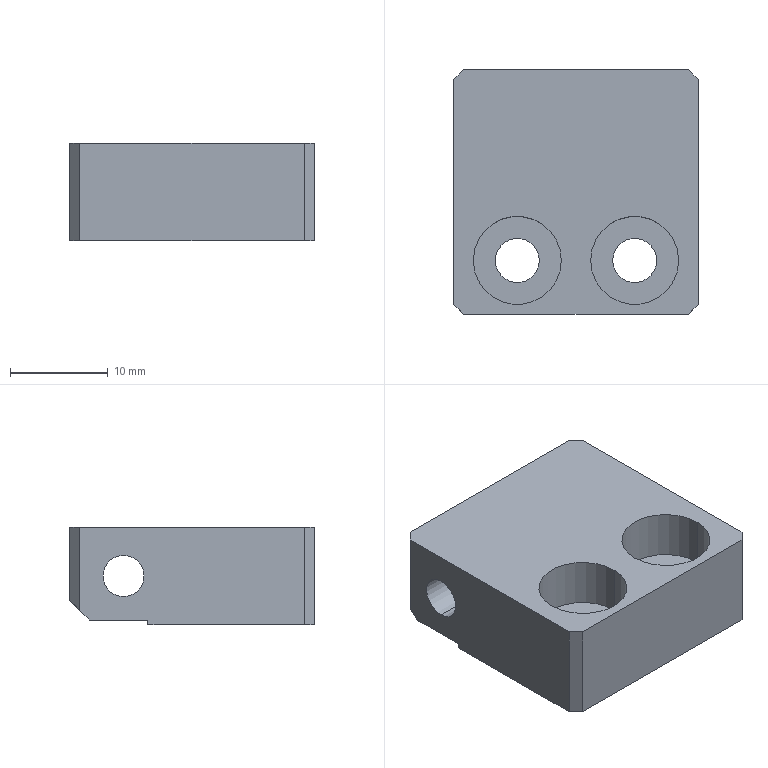Part | SolidWorks | features ICE 4, Chamfer 2, 3DProfileFeature 1, Extrusion 1, HoleWzd 1 | 1 solid | 25 faces | box 25 x 25 x 10 mm | volume 4941 mm3 | plane 15 | cylinder 10 | commonest cylinder face diameters 4.5 x4 9 x4 4.2 x2
STEP:
#1=CARTESIAN_POINT('',(12.5,7.,2.9));
#2=VERTEX_POINT('',#1);
#3=CARTESIAN_POINT('',(12.5,7.,7.1));
#4=VERTEX_POINT('',#3);
#5=CARTESIAN_POINT('',(12.5,7.,5.));
#6=DIRECTION('',(-1.,0.,0.));
#7=DIRECTION('',(0.,0.,1.));
#8=AXIS2_PLACEMENT_3D('',#5,#6,#7);
#9=CIRCLE('',#8,2.1);
#10=EDGE_CURVE('',#2,#4,#9,.T.);
#11=ORIENTED_EDGE('',*,*,#10,.F.);
#12=CARTESIAN_POINT('',(-12.5,7.,2.9));
#13=VERTEX_POINT('',#12);
#14=CARTESIAN_POINT('',(-12.5,7.,2.9));
#15=DIRECTION('',(-1.,0.,0.));
#16=VECTOR('',#15,1000.);
#17=LINE('',#14,#16);
#18=EDGE_CURVE('',#2,#13,#17,.T.);
#19=ORIENTED_EDGE('',*,*,#18,.T.);
#20=CARTESIAN_POINT('',(-12.5,7.,7.1));
#21=VERTEX_POINT('',#20);
#22=CARTESIAN_POINT('',(-12.5,7.,5.));
#23=DIRECTION('',(-1.,0.,0.));
#24=DIRECTION('',(0.,0.,1.));
#25=AXIS2_PLACEMENT_3D('',#22,#23,#24);
#26=CIRCLE('',#25,2.1);
#27=EDGE_CURVE('',#13,#21,#26,.T.);
#28=ORIENTED_EDGE('',*,*,#27,.T.);
#29=CARTESIAN_POINT('',(-12.5,7.,7.1));
#30=DIRECTION('',(-1.,0.,0.));
#31=VECTOR('',#30,1000.);
#32=LINE('',#29,#31);
#33=EDGE_CURVE('',#4,#21,#32,.T.);
#34=ORIENTED_EDGE('',*,*,#33,.F.);
#35=EDGE_LOOP('',(#11,#19,#28,#34));
#36=FACE_OUTER_BOUND('',#35,.T.);
#37=CARTESIAN_POINT('',(-12.5,7.,5.));
#38=DIRECTION('',(-1.,0.,0.));
#39=DIRECTION('',(0.,0.,1.));
#40=AXIS2_PLACEMENT_3D('',#37,#38,#39);
#41=CYLINDRICAL_SURFACE('',#40,2.1);
#42=ADVANCED_FACE('',(#36),#41,.F.);
#43=CARTESIAN_POINT('',(3.75,-7.,0.));
#44=VERTEX_POINT('',#43);
#45=CARTESIAN_POINT('',(8.25,-7.,0.));
#46=VERTEX_POINT('',#45);
#47=CARTESIAN_POINT('',(6.,-7.,0.));
#48=DIRECTION('',(0.,0.,1.));
#49=DIRECTION('',(1.,0.,0.));
#50=AXIS2_PLACEMENT_3D('',#47,#48,#49);
#51=CIRCLE('',#50,2.25);
#52=EDGE_CURVE('',#44,#46,#51,.T.);
#53=ORIENTED_EDGE('',*,*,#52,.F.);
#54=CARTESIAN_POINT('',(3.75,-7.,5.));
#55=VERTEX_POINT('',#54);
#56=CARTESIAN_POINT('',(3.75,-7.,-4.));
#57=DIRECTION('',(0.,0.,1.));
#58=VECTOR('',#57,1000.);
#59=LINE('',#56,#58);
#60=EDGE_CURVE('',#44,#55,#59,.T.);
#61=ORIENTED_EDGE('',*,*,#60,.T.);
#62=CARTESIAN_POINT('',(8.25,-7.,5.));
#63=VERTEX_POINT('',#62);
#64=CARTESIAN_POINT('',(6.,-7.,5.));
#65=DIRECTION('',(0.,0.,-1.));
#66=DIRECTION('',(-1.,0.,0.));
#67=AXIS2_PLACEMENT_3D('',#64,#65,#66);
#68=CIRCLE('',#67,2.25);
#69=EDGE_CURVE('',#63,#55,#68,.T.);
#70=ORIENTED_EDGE('',*,*,#69,.F.);
#71=CARTESIAN_POINT('',(8.25,-7.,-4.));
#72=DIRECTION('',(0.,0.,1.));
#73=VECTOR('',#72,1000.);
#74=LINE('',#71,#73);
#75=EDGE_CURVE('',#46,#63,#74,.T.);
#76=ORIENTED_EDGE('',*,*,#75,.F.);
#77=EDGE_LOOP('',(#53,#61,#70,#76));
#78=FACE_OUTER_BOUND('',#77,.T.);
#79=CARTESIAN_POINT('',(6.,-7.,-4.));
#80=DIRECTION('',(0.,0.,1.));
#81=DIRECTION('',(1.,0.,0.));
#82=AXIS2_PLACEMENT_3D('',#79,#80,#81);
#83=CYLINDRICAL_SURFACE('',#82,2.25);
#84=ADVANCED_FACE('',(#78),#83,.F.);
#85=CARTESIAN_POINT('',(-8.25,-7.,0.));
#86=VERTEX_POINT('',#85);
#87=CARTESIAN_POINT('',(-3.75,-7.,0.));
#88=VERTEX_POINT('',#87);
#89=CARTESIAN_POINT('',(-6.,-7.,0.));
#90=DIRECTION('',(0.,0.,1.));
#91=DIRECTION('',(1.,0.,0.));
#92=AXIS2_PLACEMENT_3D('',#89,#90,#91);
#93=CIRCLE('',#92,2.25);
#94=EDGE_CURVE('',#86,#88,#93,.T.);
#95=ORIENTED_EDGE('',*,*,#94,.F.);
#96=CARTESIAN_POINT('',(-8.25,-7.,5.));
#97=VERTEX_POINT('',#96);
#98=CARTESIAN_POINT('',(-8.25,-7.,-4.));
#99=DIRECTION('',(0.,0.,1.));
#100=VECTOR('',#99,1000.);
#101=LINE('',#98,#100);
#102=EDGE_CURVE('',#86,#97,#101,.T.);
#103=ORIENTED_EDGE('',*,*,#102,.T.);
#104=CARTESIAN_POINT('',(-3.75,-7.,5.));
#105=VERTEX_POINT('',#104);
#106=CARTESIAN_POINT('',(-6.,-7.,5.));
#107=DIRECTION('',(0.,0.,1.));
#108=DIRECTION('',(1.,0.,0.));
#109=AXIS2_PLACEMENT_3D('',#106,#107,#108);
#110=CIRCLE('',#109,2.25);
#111=EDGE_CURVE('',#97,#105,#110,.T.);
#112=ORIENTED_EDGE('',*,*,#111,.T.);
#113=CARTESIAN_POINT('',(-3.75,-7.,-4.));
#114=DIRECTION('',(0.,0.,1.));
#115=VECTOR('',#114,1000.);
#116=LINE('',#113,#115);
#117=EDGE_CURVE('',#88,#105,#116,.T.);
#118=ORIENTED_EDGE('',*,*,#117,.F.);
#119=EDGE_LOOP('',(#95,#103,#112,#118));
#120=FACE_OUTER_BOUND('',#119,.T.);
#121=CARTESIAN_POINT('',(-6.,-7.,-4.));
#122=DIRECTION('',(0.,0.,1.));
#123=DIRECTION('',(1.,0.,0.));
#124=AXIS2_PLACEMENT_3D('',#121,#122,#123);
#125=CYLINDRICAL_SURFACE('',#124,2.25);
#126=ADVANCED_FACE('',(#120),#125,.F.);
#127=CARTESIAN_POINT('',(1.5,-7.,5.));
#128=VERTEX_POINT('',#127);
#129=CARTESIAN_POINT('',(10.5,-7.,5.));
#130=VERTEX_POINT('',#129);
#131=CARTESIAN_POINT('',(6.,-7.,5.));
#132=DIRECTION('',(0.,0.,1.));
#133=DIRECTION('',(-1.,0.,0.));
#134=AXIS2_PLACEMENT_3D('',#131,#132,#133);
#135=CIRCLE('',#134,4.5);
#136=EDGE_CURVE('',#128,#130,#135,.T.);
#137=ORIENTED_EDGE('',*,*,#136,.F.);
#138=CARTESIAN_POINT('',(1.5,-7.,10.));
#139=VERTEX_POINT('',#138);
#140=CARTESIAN_POINT('',(1.5,-7.,5.));
#141=DIRECTION('',(0.,0.,1.));
#142=VECTOR('',#141,1000.);
#143=LINE('',#140,#142);
#144=EDGE_CURVE('',#128,#139,#143,.T.);
#145=ORIENTED_EDGE('',*,*,#144,.T.);
#146=CARTESIAN_POINT('',(10.5,-7.,10.));
#147=VERTEX_POINT('',#146);
#148=CARTESIAN_POINT('',(6.,-7.,10.));
#149=DIRECTION('',(0.,0.,1.));
#150=DIRECTION('',(-1.,0.,0.));
#151=AXIS2_PLACEMENT_3D('',#148,#149,#150);
#152=CIRCLE('',#151,4.5);
#153=EDGE_CURVE('',#139,#147,#152,.T.);
#154=ORIENTED_EDGE('',*,*,#153,.T.);
#155=CARTESIAN_POINT('',(10.5,-7.,5.));
#156=DIRECTION('',(0.,0.,1.));
#157=VECTOR('',#156,1000.);
#158=LINE('',#155,#157);
#159=EDGE_CURVE('',#130,#147,#158,.T.);
#160=ORIENTED_EDGE('',*,*,#159,.F.);
#161=EDGE_LOOP('',(#137,#145,#154,#160));
#162=FACE_OUTER_BOUND('',#161,.T.);
#163=CARTESIAN_POINT('',(6.,-7.,5.));
#164=DIRECTION('',(0.,0.,1.));
#165=DIRECTION('',(1.,0.,0.));
#166=AXIS2_PLACEMENT_3D('',#163,#164,#165);
#167=CYLINDRICAL_SURFACE('',#166,4.5);
#168=ADVANCED_FACE('',(#162),#167,.F.);
#169=CARTESIAN_POINT('',(-10.5,-7.,5.));
#170=VERTEX_POINT('',#169);
#171=CARTESIAN_POINT('',(-1.5,-7.,5.));
#172=VERTEX_POINT('',#171);
#173=CARTESIAN_POINT('',(-6.,-7.,5.));
#174=DIRECTION('',(0.,0.,1.));
#175=DIRECTION('',(1.,0.,0.));
#176=AXIS2_PLACEMENT_3D('',#173,#174,#175);
#177=CIRCLE('',#176,4.5);
#178=EDGE_CURVE('',#170,#172,#177,.T.);
#179=ORIENTED_EDGE('',*,*,#178,.F.);
#180=CARTESIAN_POINT('',(-10.5,-7.,10.));
#181=VERTEX_POINT('',#180);
#182=CARTESIAN_POINT('',(-10.5,-7.,5.));
#183=DIRECTION('',(0.,0.,1.));
#184=VECTOR('',#183,1000.);
#185=LINE('',#182,#184);
#186=EDGE_CURVE('',#170,#181,#185,.T.);
#187=ORIENTED_EDGE('',*,*,#186,.T.);
#188=CARTESIAN_POINT('',(-1.5,-7.,10.));
#189=VERTEX_POINT('',#188);
#190=CARTESIAN_POINT('',(-6.,-7.,10.));
#191=DIRECTION('',(0.,0.,1.));
#192=DIRECTION('',(1.,0.,0.));
#193=AXIS2_PLACEMENT_3D('',#190,#191,#192);
#194=CIRCLE('',#193,4.5);
#195=EDGE_CURVE('',#181,#189,#194,.T.);
#196=ORIENTED_EDGE('',*,*,#195,.T.);
#197=CARTESIAN_POINT('',(-1.5,-7.,5.));
#198=DIRECTION('',(0.,0.,1.));
#199=VECTOR('',#198,1000.);
#200=LINE('',#197,#199);
#201=EDGE_CURVE('',#172,#189,#200,.T.);
#202=ORIENTED_EDGE('',*,*,#201,.F.);
#203=EDGE_LOOP('',(#179,#187,#196,#202));
#204=FACE_OUTER_BOUND('',#203,.T.);
#205=CARTESIAN_POINT('',(-6.,-7.,5.));
#206=DIRECTION('',(0.,0.,1.));
#207=DIRECTION('',(1.,0.,0.));
#208=AXIS2_PLACEMENT_3D('',#205,#206,#207);
#209=CYLINDRICAL_SURFACE('',#208,4.5);
#210=ADVANCED_FACE('',(#204),#209,.F.);
#211=CARTESIAN_POINT('',(12.5,7.,5.));
#212=DIRECTION('',(-1.,0.,0.));
#213=DIRECTION('',(0.,0.,1.));
#214=AXIS2_PLACEMENT_3D('',#211,#212,#213);
#215=CIRCLE('',#214,2.1);
#216=EDGE_CURVE('',#4,#2,#215,.T.);
#217=ORIENTED_EDGE('',*,*,#216,.T.);
#218=ORIENTED_EDGE('',*,*,#10,.T.);
#219=EDGE_LOOP('',(#217,#218));
#220=FACE_BOUND('',#219,.T.);
#221=CARTESIAN_POINT('',(12.5,4.5,0.5));
#222=VERTEX_POINT('',#221);
#223=CARTESIAN_POINT('',(12.5,10.5,0.5));
#224=VERTEX_POINT('',#223);
#225=CARTESIAN_POINT('',(12.5,12.5,0.5));
#226=DIRECTION('',(0.,1.,0.));
#227=VECTOR('',#226,1000.);
#228=LINE('',#225,#227);
#229=EDGE_CURVE('',#222,#224,#228,.T.);
#230=ORIENTED_EDGE('',*,*,#229,.T.);
#231=CARTESIAN_POINT('',(12.5,11.5,1.5));
#232=VERTEX_POINT('',#231);
#233=CARTESIAN_POINT('',(12.5,12.5,2.5));
#234=DIRECTION('',(0.,0.7071,0.7071));
#235=VECTOR('',#234,1000.);
#236=LINE('',#233,#235);
#237=EDGE_CURVE('',#224,#232,#236,.T.);
#238=ORIENTED_EDGE('',*,*,#237,.T.);
#239=CARTESIAN_POINT('',(12.5,11.5,10.));
#240=VERTEX_POINT('',#239);
#241=CARTESIAN_POINT('',(12.5,11.5,10.));
#242=DIRECTION('',(0.,0.,1.));
#243=VECTOR('',#242,1000.);
#244=LINE('',#241,#243);
#245=EDGE_CURVE('',#232,#240,#244,.T.);
#246=ORIENTED_EDGE('',*,*,#245,.T.);
#247=CARTESIAN_POINT('',(12.5,-11.5,10.));
#248=VERTEX_POINT('',#247);
#249=CARTESIAN_POINT('',(12.5,12.5,10.));
#250=DIRECTION('',(0.,1.,0.));
#251=VECTOR('',#250,1000.);
#252=LINE('',#249,#251);
#253=EDGE_CURVE('',#248,#240,#252,.T.);
#254=ORIENTED_EDGE('',*,*,#253,.F.);
#255=CARTESIAN_POINT('',(12.5,-11.5,0.));
#256=VERTEX_POINT('',#255);
#257=CARTESIAN_POINT('',(12.5,-11.5,10.));
#258=DIRECTION('',(0.,0.,-1.));
#259=VECTOR('',#258,1000.);
#260=LINE('',#257,#259);
#261=EDGE_CURVE('',#248,#256,#260,.T.);
#262=ORIENTED_EDGE('',*,*,#261,.T.);
#263=CARTESIAN_POINT('',(12.5,4.5,0.));
#264=VERTEX_POINT('',#263);
#265=CARTESIAN_POINT('',(12.5,12.5,0.));
#266=DIRECTION('',(0.,1.,0.));
#267=VECTOR('',#266,1000.);
#268=LINE('',#265,#267);
#269=EDGE_CURVE('',#256,#264,#268,.T.);
#270=ORIENTED_EDGE('',*,*,#269,.T.);
#271=CARTESIAN_POINT('',(12.5,4.5,10.));
#272=DIRECTION('',(0.,0.,1.));
#273=VECTOR('',#272,1000.);
#274=LINE('',#271,#273);
#275=EDGE_CURVE('',#264,#222,#274,.T.);
#276=ORIENTED_EDGE('',*,*,#275,.T.);
#277=EDGE_LOOP('',(#230,#238,#246,#254,#262,#270,#276));
#278=FACE_OUTER_BOUND('',#277,.T.);
#279=CARTESIAN_POINT('',(12.5,12.5,10.));
#280=DIRECTION('',(-1.,0.,0.));
#281=DIRECTION('',(0.,-1.,0.));
#282=AXIS2_PLACEMENT_3D('',#279,#280,#281);
#283=PLANE('',#282);
#284=ADVANCED_FACE('',(#220,#278),#283,.F.);
#285=CARTESIAN_POINT('',(11.5,12.5,10.));
#286=VERTEX_POINT('',#285);
#287=CARTESIAN_POINT('',(11.5,12.5,2.5));
#288=VERTEX_POINT('',#287);
#289=CARTESIAN_POINT('',(11.5,12.5,10.));
#290=DIRECTION('',(0.,0.,-1.));
#291=VECTOR('',#290,1000.);
#292=LINE('',#289,#291);
#293=EDGE_CURVE('',#286,#288,#292,.T.);
#294=ORIENTED_EDGE('',*,*,#293,.T.);
#295=CARTESIAN_POINT('',(-11.5,12.5,2.5));
#296=VERTEX_POINT('',#295);
#297=CARTESIAN_POINT('',(-12.5,12.5,2.5));
#298=DIRECTION('',(-1.,0.,0.));
#299=VECTOR('',#298,1000.);
#300=LINE('',#297,#299);
#301=EDGE_CURVE('',#288,#296,#300,.T.);
#302=ORIENTED_EDGE('',*,*,#301,.T.);
#303=CARTESIAN_POINT('',(-11.5,12.5,10.));
#304=VERTEX_POINT('',#303);
#305=CARTESIAN_POINT('',(-11.5,12.5,10.));
#306=DIRECTION('',(0.,0.,1.));
#307=VECTOR('',#306,1000.);
#308=LINE('',#305,#307);
#309=EDGE_CURVE('',#296,#304,#308,.T.);
#310=ORIENTED_EDGE('',*,*,#309,.T.);
#311=CARTESIAN_POINT('',(-12.5,12.5,10.));
#312=DIRECTION('',(-1.,0.,0.));
#313=VECTOR('',#312,1000.);
#314=LINE('',#311,#313);
#315=EDGE_CURVE('',#286,#304,#314,.T.);
#316=ORIENTED_EDGE('',*,*,#315,.F.);
#317=EDGE_LOOP('',(#294,#302,#310,#316));
#318=FACE_OUTER_BOUND('',#317,.T.);
#319=CARTESIAN_POINT('',(-12.5,12.5,10.));
#320=DIRECTION('',(0.,-1.,0.));
#321=DIRECTION('',(0.,0.,-1.));
#322=AXIS2_PLACEMENT_3D('',#319,#320,#321);
#323=PLANE('',#322);
#324=ADVANCED_FACE('',(#318),#323,.F.);
#325=CARTESIAN_POINT('',(-12.5,7.,5.));
#326=DIRECTION('',(-1.,0.,0.));
#327=DIRECTION('',(0.,0.,1.));
#328=AXIS2_PLACEMENT_3D('',#325,#326,#327);
#329=CIRCLE('',#328,2.1);
#330=EDGE_CURVE('',#21,#13,#329,.T.);
#331=ORIENTED_EDGE('',*,*,#330,.F.);
#332=ORIENTED_EDGE('',*,*,#27,.F.);
#333=EDGE_LOOP('',(#331,#332));
#334=FACE_BOUND('',#333,.T.);
#335=CARTESIAN_POINT('',(-12.5,11.5,10.));
#336=VERTEX_POINT('',#335);
#337=CARTESIAN_POINT('',(-12.5,11.5,1.5));
#338=VERTEX_POINT('',#337);
#339=CARTESIAN_POINT('',(-12.5,11.5,10.));
#340=DIRECTION('',(0.,0.,-1.));
#341=VECTOR('',#340,1000.);
#342=LINE('',#339,#341);
#343=EDGE_CURVE('',#336,#338,#342,.T.);
#344=ORIENTED_EDGE('',*,*,#343,.T.);
#345=CARTESIAN_POINT('',(-12.5,10.5,0.5));
#346=VERTEX_POINT('',#345);
#347=CARTESIAN_POINT('',(-12.5,12.5,2.5));
#348=DIRECTION('',(0.,-0.7071,-0.7071));
#349=VECTOR('',#348,1000.);
#350=LINE('',#347,#349);
#351=EDGE_CURVE('',#338,#346,#350,.T.);
#352=ORIENTED_EDGE('',*,*,#351,.T.);
#353=CARTESIAN_POINT('',(-12.5,4.5,0.5));
#354=VERTEX_POINT('',#353);
#355=CARTESIAN_POINT('',(-12.5,12.5,0.5));
#356=DIRECTION('',(0.,1.,0.));
#357=VECTOR('',#356,1000.);
#358=LINE('',#355,#357);
#359=EDGE_CURVE('',#354,#346,#358,.T.);
#360=ORIENTED_EDGE('',*,*,#359,.F.);
#361=CARTESIAN_POINT('',(-12.5,4.5,0.));
#362=VERTEX_POINT('',#361);
#363=CARTESIAN_POINT('',(-12.5,4.5,0.));
#364=DIRECTION('',(0.,0.,1.));
#365=VECTOR('',#364,1000.);
#366=LINE('',#363,#365);
#367=EDGE_CURVE('',#362,#354,#366,.T.);
#368=ORIENTED_EDGE('',*,*,#367,.F.);
#369=CARTESIAN_POINT('',(-12.5,-11.5,0.));
#370=VERTEX_POINT('',#369);
#371=CARTESIAN_POINT('',(-12.5,12.5,0.));
#372=DIRECTION('',(0.,-1.,0.));
#373=VECTOR('',#372,1000.);
#374=LINE('',#371,#373);
#375=EDGE_CURVE('',#362,#370,#374,.T.);
#376=ORIENTED_EDGE('',*,*,#375,.T.);
#377=CARTESIAN_POINT('',(-12.5,-11.5,10.));
#378=VERTEX_POINT('',#377);
#379=CARTESIAN_POINT('',(-12.5,-11.5,10.));
#380=DIRECTION('',(0.,0.,1.));
#381=VECTOR('',#380,1000.);
#382=LINE('',#379,#381);
#383=EDGE_CURVE('',#370,#378,#382,.T.);
#384=ORIENTED_EDGE('',*,*,#383,.T.);
#385=CARTESIAN_POINT('',(-12.5,12.5,10.));
#386=DIRECTION('',(0.,-1.,0.));
#387=VECTOR('',#386,1000.);
#388=LINE('',#385,#387);
#389=EDGE_CURVE('',#336,#378,#388,.T.);
#390=ORIENTED_EDGE('',*,*,#389,.F.);
#391=EDGE_LOOP('',(#344,#352,#360,#368,#376,#384,#390));
#392=FACE_OUTER_BOUND('',#391,.T.);
#393=CARTESIAN_POINT('',(-12.5,12.5,10.));
#394=DIRECTION('',(1.,0.,0.));
#395=DIRECTION('',(0.,1.,0.));
#396=AXIS2_PLACEMENT_3D('',#393,#394,#395);
#397=PLANE('',#396);
#398=ADVANCED_FACE('',(#334,#392),#397,.F.);
#399=CARTESIAN_POINT('',(-11.5,-12.5,0.));
#400=VERTEX_POINT('',#399);
#401=CARTESIAN_POINT('',(11.5,-12.5,0.));
#402=VERTEX_POINT('',#401);
#403=CARTESIAN_POINT('',(-12.5,-12.5,0.));
#404=DIRECTION('',(1.,0.,0.));
#405=VECTOR('',#404,1000.);
#406=LINE('',#403,#405);
#407=EDGE_CURVE('',#400,#402,#406,.T.);
#408=ORIENTED_EDGE('',*,*,#407,.T.);
#409=CARTESIAN_POINT('',(11.5,-12.5,10.));
#410=VERTEX_POINT('',#409);
#411=CARTESIAN_POINT('',(11.5,-12.5,10.));
#412=DIRECTION('',(0.,0.,1.));
#413=VECTOR('',#412,1000.);
#414=LINE('',#411,#413);
#415=EDGE_CURVE('',#402,#410,#414,.T.);
#416=ORIENTED_EDGE('',*,*,#415,.T.);
#417=CARTESIAN_POINT('',(-11.5,-12.5,10.));
#418=VERTEX_POINT('',#417);
#419=CARTESIAN_POINT('',(-12.5,-12.5,10.));
#420=DIRECTION('',(1.,0.,0.));
#421=VECTOR('',#420,1000.);
#422=LINE('',#419,#421);
#423=EDGE_CURVE('',#418,#410,#422,.T.);
#424=ORIENTED_EDGE('',*,*,#423,.F.);
#425=CARTESIAN_POINT('',(-11.5,-12.5,10.));
#426=DIRECTION('',(0.,0.,-1.));
#427=VECTOR('',#426,1000.);
#428=LINE('',#425,#427);
#429=EDGE_CURVE('',#418,#400,#428,.T.);
#430=ORIENTED_EDGE('',*,*,#429,.T.);
#431=EDGE_LOOP('',(#408,#416,#424,#430));
#432=FACE_OUTER_BOUND('',#431,.T.);
#433=CARTESIAN_POINT('',(-12.5,-12.5,10.));
#434=DIRECTION('',(0.,1.,0.));
#435=DIRECTION('',(0.,0.,1.));
#436=AXIS2_PLACEMENT_3D('',#433,#434,#435);
#437=PLANE('',#436);
#438=ADVANCED_FACE('',(#432),#437,.F.);
#439=CARTESIAN_POINT('',(6.,-7.,10.));
#440=DIRECTION('',(0.,0.,1.));
#441=DIRECTION('',(-1.,0.,0.));
#442=AXIS2_PLACEMENT_3D('',#439,#440,#441);
#443=CIRCLE('',#442,4.5);
#444=EDGE_CURVE('',#147,#139,#443,.T.);
#445=ORIENTED_EDGE('',*,*,#444,.F.);
#446=ORIENTED_EDGE('',*,*,#153,.F.);
#447=EDGE_LOOP('',(#445,#446));
#448=FACE_BOUND('',#447,.T.);
#449=CARTESIAN_POINT('',(-6.,-7.,10.));
#450=DIRECTION('',(0.,0.,1.));
#451=DIRECTION('',(1.,0.,0.));
#452=AXIS2_PLACEMENT_3D('',#449,#450,#451);
#453=CIRCLE('',#452,4.5);
#454=EDGE_CURVE('',#189,#181,#453,.T.);
#455=ORIENTED_EDGE('',*,*,#454,.F.);
#456=ORIENTED_EDGE('',*,*,#195,.F.);
#457=EDGE_LOOP('',(#455,#456));
#458=FACE_BOUND('',#457,.T.);
#459=ORIENTED_EDGE('',*,*,#423,.T.);
#460=CARTESIAN_POINT('',(12.,-12.,10.));
#461=DIRECTION('',(0.7071,0.7071,0.));
#462=VECTOR('',#461,1000.);
#463=LINE('',#460,#462);
#464=EDGE_CURVE('',#410,#248,#463,.T.);
#465=ORIENTED_EDGE('',*,*,#464,.T.);
#466=ORIENTED_EDGE('',*,*,#253,.T.);
#467=CARTESIAN_POINT('',(12.,12.,10.));
#468=DIRECTION('',(-0.7071,0.7071,0.));
#469=VECTOR('',#468,1000.);
#470=LINE('',#467,#469);
#471=EDGE_CURVE('',#240,#286,#470,.T.);
#472=ORIENTED_EDGE('',*,*,#471,.T.);
#473=ORIENTED_EDGE('',*,*,#315,.T.);
#474=CARTESIAN_POINT('',(-12.,12.,10.));
#475=DIRECTION('',(-0.7071,-0.7071,0.));
#476=VECTOR('',#475,1000.);
#477=LINE('',#474,#476);
#478=EDGE_CURVE('',#304,#336,#477,.T.);
#479=ORIENTED_EDGE('',*,*,#478,.T.);
#480=ORIENTED_EDGE('',*,*,#389,.T.);
#481=CARTESIAN_POINT('',(-12.,-12.,10.));
#482=DIRECTION('',(0.7071,-0.7071,0.));
#483=VECTOR('',#482,1000.);
#484=LINE('',#481,#483);
#485=EDGE_CURVE('',#378,#418,#484,.T.);
#486=ORIENTED_EDGE('',*,*,#485,.T.);
#487=EDGE_LOOP('',(#459,#465,#466,#472,#473,#479,#480,#486));
#488=FACE_OUTER_BOUND('',#487,.T.);
#489=CARTESIAN_POINT('',(0.,0.,10.));
#490=DIRECTION('',(0.,0.,1.));
#491=DIRECTION('',(1.,0.,0.));
#492=AXIS2_PLACEMENT_3D('',#489,#490,#491);
#493=PLANE('',#492);
#494=ADVANCED_FACE('',(#448,#458,#488),#493,.T.);
#495=CARTESIAN_POINT('',(6.,-7.,0.));
#496=DIRECTION('',(0.,0.,1.));
#497=DIRECTION('',(1.,0.,0.));
#498=AXIS2_PLACEMENT_3D('',#495,#496,#497);
#499=CIRCLE('',#498,2.25);
#500=EDGE_CURVE('',#46,#44,#499,.T.);
#501=ORIENTED_EDGE('',*,*,#500,.T.);
#502=ORIENTED_EDGE('',*,*,#52,.T.);
#503=EDGE_LOOP('',(#501,#502));
#504=FACE_BOUND('',#503,.T.);
#505=CARTESIAN_POINT('',(-6.,-7.,0.));
#506=DIRECTION('',(0.,0.,1.));
#507=DIRECTION('',(1.,0.,0.));
#508=AXIS2_PLACEMENT_3D('',#505,#506,#507);
#509=CIRCLE('',#508,2.25);
#510=EDGE_CURVE('',#88,#86,#509,.T.);
#511=ORIENTED_EDGE('',*,*,#510,.T.);
#512=ORIENTED_EDGE('',*,*,#94,.T.);
#513=EDGE_LOOP('',(#511,#512));
#514=FACE_BOUND('',#513,.T.);
#515=ORIENTED_EDGE('',*,*,#375,.F.);
#516=CARTESIAN_POINT('',(18.5,4.5,0.));
#517=DIRECTION('',(-1.,0.,0.));
#518=VECTOR('',#517,1000.);
#519=LINE('',#516,#518);
#520=EDGE_CURVE('',#264,#362,#519,.T.);
#521=ORIENTED_EDGE('',*,*,#520,.F.);
#522=ORIENTED_EDGE('',*,*,#269,.F.);
#523=CARTESIAN_POINT('',(12.5,-11.5,0.));
#524=DIRECTION('',(-0.7071,-0.7071,0.));
#525=VECTOR('',#524,1000.);
#526=LINE('',#523,#525);
#527=EDGE_CURVE('',#256,#402,#526,.T.);
#528=ORIENTED_EDGE('',*,*,#527,.T.);
#529=ORIENTED_EDGE('',*,*,#407,.F.);
#530=CARTESIAN_POINT('',(-11.5,-12.5,0.));
#531=DIRECTION('',(-0.7071,0.7071,0.));
#532=VECTOR('',#531,1000.);
#533=LINE('',#530,#532);
#534=EDGE_CURVE('',#400,#370,#533,.T.);
#535=ORIENTED_EDGE('',*,*,#534,.T.);
#536=EDGE_LOOP('',(#515,#521,#522,#528,#529,#535));
#537=FACE_OUTER_BOUND('',#536,.T.);
#538=CARTESIAN_POINT('',(0.,0.,0.));
#539=DIRECTION('',(0.,0.,1.));
#540=DIRECTION('',(1.,0.,0.));
#541=AXIS2_PLACEMENT_3D('',#538,#539,#540);
#542=PLANE('',#541);
#543=ADVANCED_FACE('',(#504,#514,#537),#542,.F.);
#544=ORIENTED_EDGE('',*,*,#186,.F.);
#545=CARTESIAN_POINT('',(-6.,-7.,5.));
#546=DIRECTION('',(0.,0.,1.));
#547=DIRECTION('',(1.,0.,0.));
#548=AXIS2_PLACEMENT_3D('',#545,#546,#547);
#549=CIRCLE('',#548,4.5);
#550=EDGE_CURVE('',#172,#170,#549,.T.);
#551=ORIENTED_EDGE('',*,*,#550,.F.);
#552=ORIENTED_EDGE('',*,*,#201,.T.);
#553=ORIENTED_EDGE('',*,*,#454,.T.);
#554=EDGE_LOOP('',(#544,#551,#552,#553));
#555=FACE_OUTER_BOUND('',#554,.T.);
#556=CARTESIAN_POINT('',(-6.,-7.,5.));
#557=DIRECTION('',(0.,0.,1.));
#558=DIRECTION('',(1.,0.,0.));
#559=AXIS2_PLACEMENT_3D('',#556,#557,#558);
#560=CYLINDRICAL_SURFACE('',#559,4.5);
#561=ADVANCED_FACE('',(#555),#560,.F.);
#562=CARTESIAN_POINT('',(-6.,-7.,5.));
#563=DIRECTION('',(0.,0.,1.));
#564=DIRECTION('',(1.,0.,0.));
#565=AXIS2_PLACEMENT_3D('',#562,#563,#564);
#566=CIRCLE('',#565,2.25);
#567=EDGE_CURVE('',#105,#97,#566,.T.);
#568=ORIENTED_EDGE('',*,*,#567,.F.);
#569=ORIENTED_EDGE('',*,*,#111,.F.);
#570=EDGE_LOOP('',(#568,#569));
#571=FACE_BOUND('',#570,.T.);
#572=ORIENTED_EDGE('',*,*,#550,.T.);
#573=ORIENTED_EDGE('',*,*,#178,.T.);
#574=EDGE_LOOP('',(#572,#573));
#575=FACE_OUTER_BOUND('',#574,.T.);
#576=CARTESIAN_POINT('',(-6.,-7.,5.));
#577=DIRECTION('',(0.,0.,1.));
#578=DIRECTION('',(1.,0.,0.));
#579=AXIS2_PLACEMENT_3D('',#576,#577,#578);
#580=PLANE('',#579);
#581=ADVANCED_FACE('',(#571,#575),#580,.T.);
#582=ORIENTED_EDGE('',*,*,#144,.F.);
#583=CARTESIAN_POINT('',(6.,-7.,5.));
#584=DIRECTION('',(0.,0.,1.));
#585=DIRECTION('',(-1.,0.,0.));
#586=AXIS2_PLACEMENT_3D('',#583,#584,#585);
#587=CIRCLE('',#586,4.5);
#588=EDGE_CURVE('',#130,#128,#587,.T.);
#589=ORIENTED_EDGE('',*,*,#588,.F.);
#590=ORIENTED_EDGE('',*,*,#159,.T.);
#591=ORIENTED_EDGE('',*,*,#444,.T.);
#592=EDGE_LOOP('',(#582,#589,#590,#591));
#593=FACE_OUTER_BOUND('',#592,.T.);
#594=CARTESIAN_POINT('',(6.,-7.,5.));
#595=DIRECTION('',(0.,0.,1.));
#596=DIRECTION('',(1.,0.,0.));
#597=AXIS2_PLACEMENT_3D('',#594,#595,#596);
#598=CYLINDRICAL_SURFACE('',#597,4.5);
#599=ADVANCED_FACE('',(#593),#598,.F.);
#600=ORIENTED_EDGE('',*,*,#69,.T.);
#601=CARTESIAN_POINT('',(6.,-7.,5.));
#602=DIRECTION('',(0.,0.,-1.));
#603=DIRECTION('',(-1.,0.,0.));
#604=AXIS2_PLACEMENT_3D('',#601,#602,#603);
#605=CIRCLE('',#604,2.25);
#606=EDGE_CURVE('',#55,#63,#605,.T.);
#607=ORIENTED_EDGE('',*,*,#606,.T.);
#608=EDGE_LOOP('',(#600,#607));
#609=FACE_BOUND('',#608,.T.);
#610=ORIENTED_EDGE('',*,*,#588,.T.);
#611=ORIENTED_EDGE('',*,*,#136,.T.);
#612=EDGE_LOOP('',(#610,#611));
#613=FACE_OUTER_BOUND('',#612,.T.);
#614=CARTESIAN_POINT('',(6.,-7.,5.));
#615=DIRECTION('',(0.,0.,-1.));
#616=DIRECTION('',(-1.,0.,0.));
#617=AXIS2_PLACEMENT_3D('',#614,#615,#616);
#618=PLANE('',#617);
#619=ADVANCED_FACE('',(#609,#613),#618,.F.);
#620=ORIENTED_EDGE('',*,*,#102,.F.);
#621=ORIENTED_EDGE('',*,*,#510,.F.);
#622=ORIENTED_EDGE('',*,*,#117,.T.);
#623=ORIENTED_EDGE('',*,*,#567,.T.);
#624=EDGE_LOOP('',(#620,#621,#622,#623));
#625=FACE_OUTER_BOUND('',#624,.T.);
#626=CARTESIAN_POINT('',(-6.,-7.,-4.));
#627=DIRECTION('',(0.,0.,1.));
#628=DIRECTION('',(1.,0.,0.));
#629=AXIS2_PLACEMENT_3D('',#626,#627,#628);
#630=CYLINDRICAL_SURFACE('',#629,2.25);
#631=ADVANCED_FACE('',(#625),#630,.F.);
#632=ORIENTED_EDGE('',*,*,#60,.F.);
#633=ORIENTED_EDGE('',*,*,#500,.F.);
#634=ORIENTED_EDGE('',*,*,#75,.T.);
#635=ORIENTED_EDGE('',*,*,#606,.F.);
#636=EDGE_LOOP('',(#632,#633,#634,#635));
#637=FACE_OUTER_BOUND('',#636,.T.);
#638=CARTESIAN_POINT('',(6.,-7.,-4.));
#639=DIRECTION('',(0.,0.,1.));
#640=DIRECTION('',(1.,0.,0.));
#641=AXIS2_PLACEMENT_3D('',#638,#639,#640);
#642=CYLINDRICAL_SURFACE('',#641,2.25);
#643=ADVANCED_FACE('',(#637),#642,.F.);
#644=ORIENTED_EDGE('',*,*,#18,.F.);
#645=ORIENTED_EDGE('',*,*,#216,.F.);
#646=ORIENTED_EDGE('',*,*,#33,.T.);
#647=ORIENTED_EDGE('',*,*,#330,.T.);
#648=EDGE_LOOP('',(#644,#645,#646,#647));
#649=FACE_OUTER_BOUND('',#648,.T.);
#650=CARTESIAN_POINT('',(-12.5,7.,5.));
#651=DIRECTION('',(-1.,0.,0.));
#652=DIRECTION('',(0.,0.,1.));
#653=AXIS2_PLACEMENT_3D('',#650,#651,#652);
#654=CYLINDRICAL_SURFACE('',#653,2.1);
#655=ADVANCED_FACE('',(#649),#654,.F.);
#656=ORIENTED_EDGE('',*,*,#464,.F.);
#657=ORIENTED_EDGE('',*,*,#415,.F.);
#658=ORIENTED_EDGE('',*,*,#527,.F.);
#659=ORIENTED_EDGE('',*,*,#261,.F.);
#660=EDGE_LOOP('',(#656,#657,#658,#659));
#661=FACE_OUTER_BOUND('',#660,.T.);
#662=CARTESIAN_POINT('',(12.5,-11.5,10.));
#663=DIRECTION('',(-0.7071,0.7071,0.));
#664=DIRECTION('',(0.,0.,-1.));
#665=AXIS2_PLACEMENT_3D('',#662,#663,#664);
#666=PLANE('',#665);
#667=ADVANCED_FACE('',(#661),#666,.F.);
#668=ORIENTED_EDGE('',*,*,#485,.F.);
#669=ORIENTED_EDGE('',*,*,#383,.F.);
#670=ORIENTED_EDGE('',*,*,#534,.F.);
#671=ORIENTED_EDGE('',*,*,#429,.F.);
#672=EDGE_LOOP('',(#668,#669,#670,#671));
#673=FACE_OUTER_BOUND('',#672,.T.);
#674=CARTESIAN_POINT('',(-11.5,-12.5,10.));
#675=DIRECTION('',(0.7071,0.7071,0.));
#676=DIRECTION('',(0.,0.,-1.));
#677=AXIS2_PLACEMENT_3D('',#674,#675,#676);
#678=PLANE('',#677);
#679=ADVANCED_FACE('',(#673),#678,.F.);
#680=ORIENTED_EDGE('',*,*,#245,.F.);
#681=CARTESIAN_POINT('',(9.,15.,5.));
#682=DIRECTION('',(-0.5774,0.5774,0.5774));
#683=VECTOR('',#682,1000.);
#684=LINE('',#681,#683);
#685=EDGE_CURVE('',#232,#288,#684,.T.);
#686=ORIENTED_EDGE('',*,*,#685,.T.);
#687=ORIENTED_EDGE('',*,*,#293,.F.);
#688=ORIENTED_EDGE('',*,*,#471,.F.);
#689=EDGE_LOOP('',(#680,#686,#687,#688));
#690=FACE_OUTER_BOUND('',#689,.T.);
#691=CARTESIAN_POINT('',(11.5,12.5,10.));
#692=DIRECTION('',(-0.7071,-0.7071,0.));
#693=DIRECTION('',(0.,0.,-1.));
#694=AXIS2_PLACEMENT_3D('',#691,#692,#693);
#695=PLANE('',#694);
#696=ADVANCED_FACE('',(#690),#695,.F.);
#697=ORIENTED_EDGE('',*,*,#309,.F.);
#698=CARTESIAN_POINT('',(-9.667,14.333,4.333));
#699=DIRECTION('',(-0.5774,-0.5774,-0.5774));
#700=VECTOR('',#699,1000.);
#701=LINE('',#698,#700);
#702=EDGE_CURVE('',#296,#338,#701,.T.);
#703=ORIENTED_EDGE('',*,*,#702,.T.);
#704=ORIENTED_EDGE('',*,*,#343,.F.);
#705=ORIENTED_EDGE('',*,*,#478,.F.);
#706=EDGE_LOOP('',(#697,#703,#704,#705));
#707=FACE_OUTER_BOUND('',#706,.T.);
#708=CARTESIAN_POINT('',(-12.5,11.5,10.));
#709=DIRECTION('',(0.7071,-0.7071,0.));
#710=DIRECTION('',(0.,0.,-1.));
#711=AXIS2_PLACEMENT_3D('',#708,#709,#710);
#712=PLANE('',#711);
#713=ADVANCED_FACE('',(#707),#712,.F.);
#714=ORIENTED_EDGE('',*,*,#520,.T.);
#715=ORIENTED_EDGE('',*,*,#367,.T.);
#716=CARTESIAN_POINT('',(18.5,4.5,0.5));
#717=DIRECTION('',(-1.,0.,0.));
#718=VECTOR('',#717,1000.);
#719=LINE('',#716,#718);
#720=EDGE_CURVE('',#222,#354,#719,.T.);
#721=ORIENTED_EDGE('',*,*,#720,.F.);
#722=ORIENTED_EDGE('',*,*,#275,.F.);
#723=EDGE_LOOP('',(#714,#715,#721,#722));
#724=FACE_OUTER_BOUND('',#723,.T.);
#725=CARTESIAN_POINT('',(18.5,4.5,0.));
#726=DIRECTION('',(0.,-1.,0.));
#727=DIRECTION('',(1.,0.,0.));
#728=AXIS2_PLACEMENT_3D('',#725,#726,#727);
#729=PLANE('',#728);
#730=ADVANCED_FACE('',(#724),#729,.F.);
#731=ORIENTED_EDGE('',*,*,#359,.T.);
#732=CARTESIAN_POINT('',(18.5,10.5,0.5));
#733=DIRECTION('',(1.,0.,0.));
#734=VECTOR('',#733,1000.);
#735=LINE('',#732,#734);
#736=EDGE_CURVE('',#346,#224,#735,.T.);
#737=ORIENTED_EDGE('',*,*,#736,.T.);
#738=ORIENTED_EDGE('',*,*,#229,.F.);
#739=ORIENTED_EDGE('',*,*,#720,.T.);
#740=EDGE_LOOP('',(#731,#737,#738,#739));
#741=FACE_OUTER_BOUND('',#740,.T.);
#742=CARTESIAN_POINT('',(18.5,12.5,0.5));
#743=DIRECTION('',(0.,0.,1.));
#744=DIRECTION('',(0.,-1.,0.));
#745=AXIS2_PLACEMENT_3D('',#742,#743,#744);
#746=PLANE('',#745);
#747=ADVANCED_FACE('',(#741),#746,.F.);
#748=ORIENTED_EDGE('',*,*,#237,.F.);
#749=ORIENTED_EDGE('',*,*,#736,.F.);
#750=ORIENTED_EDGE('',*,*,#351,.F.);
#751=ORIENTED_EDGE('',*,*,#702,.F.);
#752=ORIENTED_EDGE('',*,*,#301,.F.);
#753=ORIENTED_EDGE('',*,*,#685,.F.);
#754=EDGE_LOOP('',(#748,#749,#750,#751,#752,#753));
#755=FACE_OUTER_BOUND('',#754,.T.);
#756=CARTESIAN_POINT('',(-12.5,12.5,2.5));
#757=DIRECTION('',(0.,-0.7071,0.7071));
#758=DIRECTION('',(-1.,0.,0.));
#759=AXIS2_PLACEMENT_3D('',#756,#757,#758);
#760=PLANE('',#759);
#761=ADVANCED_FACE('',(#755),#760,.F.);
#762=CLOSED_SHELL('',(#42,#84,#126,#168,#210,#284,#324,#398,#438,#494,#543,#561,#581,#599,#619,#631,#643,#655,#667,#679,#696,#713,#730,#747,#761));
#763=MANIFOLD_SOLID_BREP('',#762);
#764=CARTESIAN_POINT('',(0.,0.,0.));
#765=DIRECTION('',(0.,0.,1.));
#766=DIRECTION('',(1.,0.,0.));
#767=AXIS2_PLACEMENT_3D('',#764,#765,#766);
#768=(LENGTH_UNIT()NAMED_UNIT(*)SI_UNIT(.MILLI.,.METRE.));
#769=UNCERTAINTY_MEASURE_WITH_UNIT(LENGTH_MEASURE(0.00001),#768,'','');
#770=(NAMED_UNIT(*)PLANE_ANGLE_UNIT()SI_UNIT($,.RADIAN.));
#771=(NAMED_UNIT(*)SI_UNIT($,.STERADIAN.)SOLID_ANGLE_UNIT());
#772=(GEOMETRIC_REPRESENTATION_CONTEXT(3)GLOBAL_UNCERTAINTY_ASSIGNED_CONTEXT((#769))GLOBAL_UNIT_ASSIGNED_CONTEXT((#768,#770,#771))REPRESENTATION_CONTEXT('',''));
#773=ADVANCED_BREP_SHAPE_REPRESENTATION('',(#763,#767),#772);